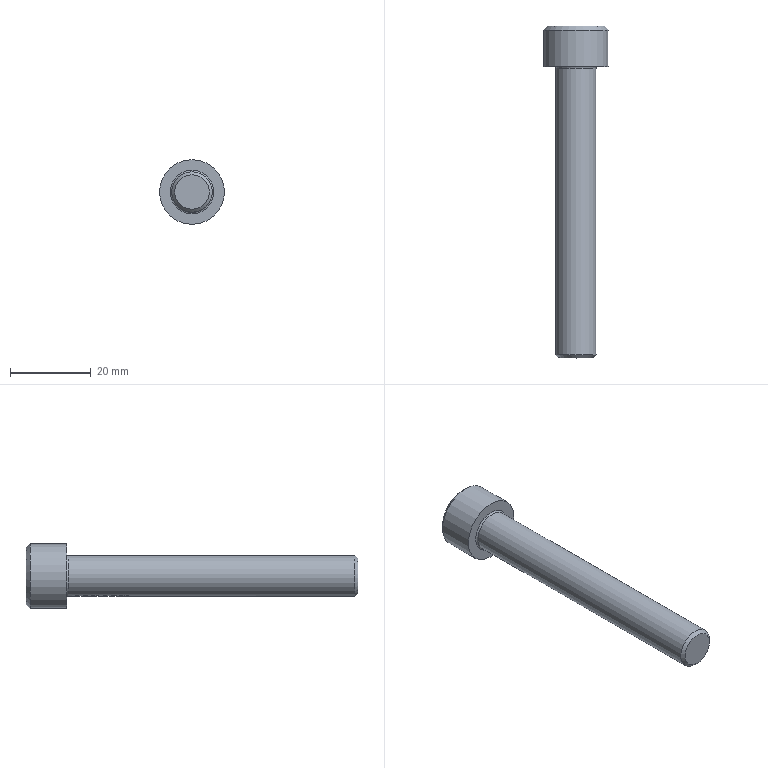Part | STEP file | solid 51 | 1 solid | 112 faces | box 16 x 82 x 16 mm | volume 7351 mm3 | plane 58 | other 37 | cylinder 8 | sphere 6 | cone 2 | torus 1 | commonest cylinder face diameters 10 x7 16 x1